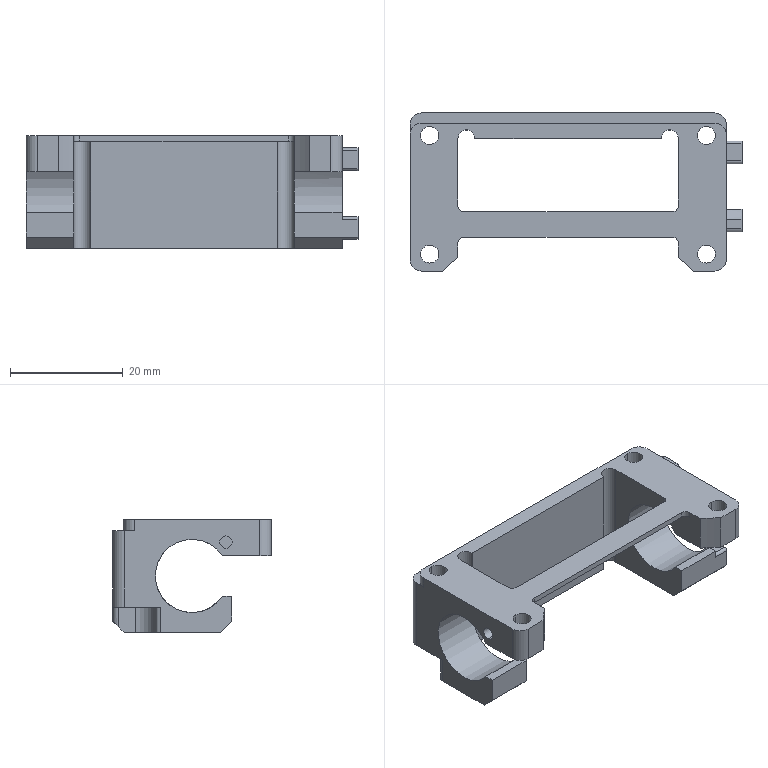NC program | Mastercam | posted with a generic post | part box 58.8 x 28 x 20 mm
Lines 1 to 57 of 29451:
%
:0001()
(MATERIAL - ALUMINUM MM - 2024)
(T24|100 FEM |H24)
(T7|4 CHM |H7)
(T1|3 DR |H1)
(T10|10 FEM |H10|XY STOCK TO LEAVE - .1|Z STOCK TO LEAVE - 0.)
(T6|6 FEM |H6)
(T3|3 FEM |H3)
(T18|8 BNOS |H18)
(T2|2 FEM |H2)
(T5|4 CHM |H5)
(T9|10 FEM |H9|XY STOCK TO LEAVE - .1|Z STOCK TO LEAVE - 0.)
N100 G21
N102 G0 G17 G40 G80 G90 G94 G98
N104 G0 G28 G91 Z0.
N106 G0 G28 X0. Y0.
(100 FEM |TOOL - 24|DIA. OFF. - 24|LEN. - 24|TOOL DIA. - 100.)
N108 T24 M6
N110 G0 G54 G90 X-114.5 Y0. C0. B0. S4000 M3
N112 G43 H24 Z25.
N114 Z1.
N116 G1 Z0. F600.
N118 X114.5 F1000.
N120 G0 Z25.
N122 M5
N124 G0 G28 G91 Z0.
N126 G28
N128 M01
N130 G0 G17 G40 G80 G90 G94 G98
N132 G0 G28 G91 Z0.
(4 CHM |TOOL - 7|DIA. OFF. - 7|LEN. - 7|TOOL DIA. - 4.)
N134 T7 M6
N136 G0 G54 G90 X-16.635 Y9.5 C0. B0. S3000 M3
N138 G43 H7 Z50.
N140 G81 G98 Z-.7 R1. F300.
N142 X19.435
N144 G80
N146 M5
N148 G0 G28 G91 Z0.
N150 G28
N152 M01
N154 G0 G17 G40 G80 G90 G94 G98
N156 G0 G28 G91 Z0.
(3 DR |TOOL - 1|DIA. OFF. - 1|LEN. - 1|TOOL DIA. - 3.)
N158 T1 M6
N160 G0 G54 G90 X-16.635 Y9.5 C0. B0. S1200 M3
N162 G43 H1 Z50.
N164 G83 G98 Z-23. R1. Q2. F100.
N166 X19.435
N168 G80
N170 M5
N172 G0 G28 G91 Z0.
N174 G28
N176 M01
N178 G0 G17 G40 G80 G90 G94 G98
N180 G0 G28 G91 Z0.